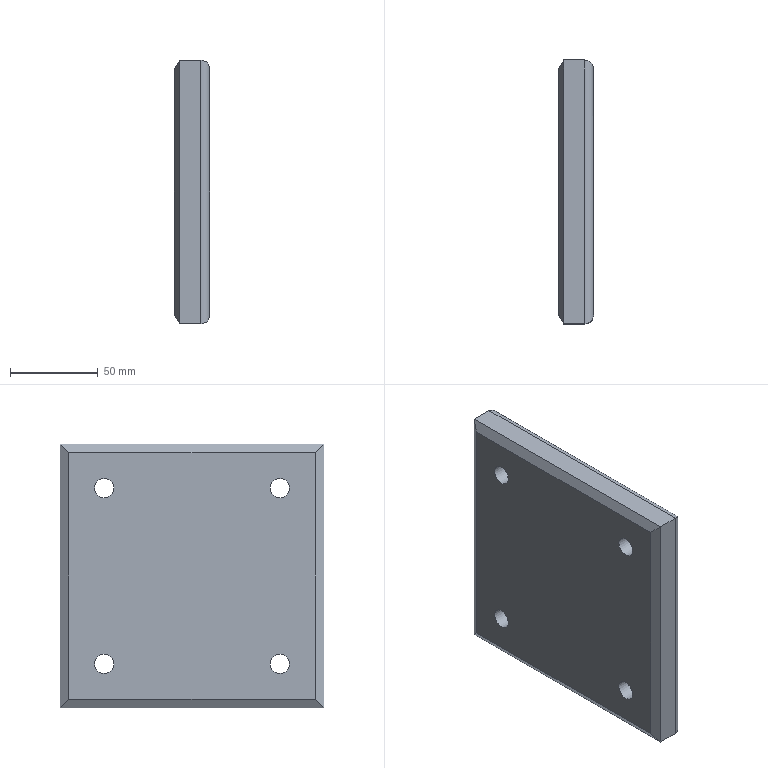Part | NX | features solid 2 | 1 solid | 30 faces | box 20 x 150 x 150 mm | volume 427385 mm3 | plane 14 | cylinder 12 | torus 4 | commonest cylinder face diameters 10 x4 11 x4 17.5 x4
STEP:
#1=CARTESIAN_POINT('',(715.,-50.,-145.));
#2=VERTEX_POINT('',#1);
#3=CARTESIAN_POINT('',(715.,-50.,-285.));
#4=VERTEX_POINT('',#3);
#5=CARTESIAN_POINT('',(715.,-50.,-290.));
#6=DIRECTION('',(0.,0.,-1.));
#7=VECTOR('',#6,1000.);
#8=LINE('',#5,#7);
#9=EDGE_CURVE('',#2,#4,#8,.T.);
#10=ORIENTED_EDGE('',*,*,#9,.F.);
#11=CARTESIAN_POINT('',(715.,-190.,-145.));
#12=VERTEX_POINT('',#11);
#13=CARTESIAN_POINT('',(715.,-195.,-145.));
#14=DIRECTION('',(0.,1.,0.));
#15=VECTOR('',#14,1000.);
#16=LINE('',#13,#15);
#17=EDGE_CURVE('',#12,#2,#16,.T.);
#18=ORIENTED_EDGE('',*,*,#17,.F.);
#19=CARTESIAN_POINT('',(715.,-190.,-285.));
#20=VERTEX_POINT('',#19);
#21=CARTESIAN_POINT('',(715.,-190.,-140.));
#22=DIRECTION('',(0.,0.,1.));
#23=VECTOR('',#22,1000.);
#24=LINE('',#21,#23);
#25=EDGE_CURVE('',#20,#12,#24,.T.);
#26=ORIENTED_EDGE('',*,*,#25,.F.);
#27=CARTESIAN_POINT('',(715.,-195.,-285.));
#28=DIRECTION('',(0.,-1.,0.));
#29=VECTOR('',#28,1000.);
#30=LINE('',#27,#29);
#31=EDGE_CURVE('',#4,#20,#30,.T.);
#32=ORIENTED_EDGE('',*,*,#31,.F.);
#33=EDGE_LOOP('',(#10,#18,#26,#32));
#34=FACE_BOUND('',#33,.T.);
#35=CARTESIAN_POINT('',(715.,-70.,-153.25));
#36=VERTEX_POINT('',#35);
#37=CARTESIAN_POINT('',(715.,-70.,-165.));
#38=DIRECTION('',(1.,0.,0.));
#39=DIRECTION('',(0.,0.,1.));
#40=AXIS2_PLACEMENT_3D('',#37,#38,#39);
#41=CIRCLE('',#40,11.75);
#42=EDGE_CURVE('',#36,#36,#41,.T.);
#43=ORIENTED_EDGE('',*,*,#42,.F.);
#44=EDGE_LOOP('',(#43));
#45=FACE_BOUND('',#44,.T.);
#46=CARTESIAN_POINT('',(715.,-70.,-253.25));
#47=VERTEX_POINT('',#46);
#48=CARTESIAN_POINT('',(715.,-70.,-265.));
#49=DIRECTION('',(1.,0.,0.));
#50=DIRECTION('',(0.,0.,1.));
#51=AXIS2_PLACEMENT_3D('',#48,#49,#50);
#52=CIRCLE('',#51,11.75);
#53=EDGE_CURVE('',#47,#47,#52,.T.);
#54=ORIENTED_EDGE('',*,*,#53,.F.);
#55=EDGE_LOOP('',(#54));
#56=FACE_BOUND('',#55,.T.);
#57=CARTESIAN_POINT('',(715.,-170.,-253.25));
#58=VERTEX_POINT('',#57);
#59=CARTESIAN_POINT('',(715.,-170.,-265.));
#60=DIRECTION('',(1.,0.,0.));
#61=DIRECTION('',(0.,0.,1.));
#62=AXIS2_PLACEMENT_3D('',#59,#60,#61);
#63=CIRCLE('',#62,11.75);
#64=EDGE_CURVE('',#58,#58,#63,.T.);
#65=ORIENTED_EDGE('',*,*,#64,.F.);
#66=EDGE_LOOP('',(#65));
#67=FACE_BOUND('',#66,.T.);
#68=CARTESIAN_POINT('',(715.,-170.,-153.25));
#69=VERTEX_POINT('',#68);
#70=CARTESIAN_POINT('',(715.,-170.,-165.));
#71=DIRECTION('',(1.,0.,0.));
#72=DIRECTION('',(0.,0.,1.));
#73=AXIS2_PLACEMENT_3D('',#70,#71,#72);
#74=CIRCLE('',#73,11.75);
#75=EDGE_CURVE('',#69,#69,#74,.T.);
#76=ORIENTED_EDGE('',*,*,#75,.F.);
#77=EDGE_LOOP('',(#76));
#78=FACE_BOUND('',#77,.T.);
#79=CARTESIAN_POINT('',(715.,-195.,-290.));
#80=DIRECTION('',(1.,0.,0.));
#81=DIRECTION('',(0.,0.,-1.));
#82=AXIS2_PLACEMENT_3D('',#79,#80,#81);
#83=PLANE('',#82);
#84=ADVANCED_FACE('',(#34,#45,#56,#67,#78),#83,.T.);
#85=CARTESIAN_POINT('',(710.,-195.,-140.));
#86=VERTEX_POINT('',#85);
#87=CARTESIAN_POINT('',(698.,-195.,-140.));
#88=VERTEX_POINT('',#87);
#89=CARTESIAN_POINT('',(715.,-195.,-140.));
#90=DIRECTION('',(-1.,0.,0.));
#91=VECTOR('',#90,1000.);
#92=LINE('',#89,#91);
#93=EDGE_CURVE('',#86,#88,#92,.T.);
#94=ORIENTED_EDGE('',*,*,#93,.F.);
#95=CARTESIAN_POINT('',(710.,-45.,-140.));
#96=VERTEX_POINT('',#95);
#97=CARTESIAN_POINT('',(710.,-195.,-140.));
#98=DIRECTION('',(0.,-1.,0.));
#99=VECTOR('',#98,1000.);
#100=LINE('',#97,#99);
#101=EDGE_CURVE('',#96,#86,#100,.T.);
#102=ORIENTED_EDGE('',*,*,#101,.F.);
#103=CARTESIAN_POINT('',(698.,-45.,-140.));
#104=VERTEX_POINT('',#103);
#105=CARTESIAN_POINT('',(715.,-45.,-140.));
#106=DIRECTION('',(-1.,0.,0.));
#107=VECTOR('',#106,1000.);
#108=LINE('',#105,#107);
#109=EDGE_CURVE('',#96,#104,#108,.T.);
#110=ORIENTED_EDGE('',*,*,#109,.T.);
#111=CARTESIAN_POINT('',(698.,-195.,-140.));
#112=DIRECTION('',(0.,1.,0.));
#113=VECTOR('',#112,1000.);
#114=LINE('',#111,#113);
#115=EDGE_CURVE('',#88,#104,#114,.T.);
#116=ORIENTED_EDGE('',*,*,#115,.F.);
#117=EDGE_LOOP('',(#94,#102,#110,#116));
#118=FACE_BOUND('',#117,.T.);
#119=CARTESIAN_POINT('',(715.,-195.,-140.));
#120=DIRECTION('',(0.,0.,1.));
#121=DIRECTION('',(1.,0.,0.));
#122=AXIS2_PLACEMENT_3D('',#119,#120,#121);
#123=PLANE('',#122);
#124=ADVANCED_FACE('',(#118),#123,.T.);
#125=CARTESIAN_POINT('',(695.,-190.,-145.));
#126=VERTEX_POINT('',#125);
#127=CARTESIAN_POINT('',(695.,-190.,-285.));
#128=VERTEX_POINT('',#127);
#129=CARTESIAN_POINT('',(695.,-190.,-290.));
#130=DIRECTION('',(0.,0.,-1.));
#131=VECTOR('',#130,1000.);
#132=LINE('',#129,#131);
#133=EDGE_CURVE('',#126,#128,#132,.T.);
#134=ORIENTED_EDGE('',*,*,#133,.F.);
#135=CARTESIAN_POINT('',(695.,-50.,-145.));
#136=VERTEX_POINT('',#135);
#137=CARTESIAN_POINT('',(695.,-195.,-145.));
#138=DIRECTION('',(0.,-1.,0.));
#139=VECTOR('',#138,1000.);
#140=LINE('',#137,#139);
#141=EDGE_CURVE('',#136,#126,#140,.T.);
#142=ORIENTED_EDGE('',*,*,#141,.F.);
#143=CARTESIAN_POINT('',(695.,-50.,-285.));
#144=VERTEX_POINT('',#143);
#145=CARTESIAN_POINT('',(695.,-50.,-290.));
#146=DIRECTION('',(0.,0.,1.));
#147=VECTOR('',#146,1000.);
#148=LINE('',#145,#147);
#149=EDGE_CURVE('',#144,#136,#148,.T.);
#150=ORIENTED_EDGE('',*,*,#149,.F.);
#151=CARTESIAN_POINT('',(695.,-195.,-285.));
#152=DIRECTION('',(0.,1.,0.));
#153=VECTOR('',#152,1000.);
#154=LINE('',#151,#153);
#155=EDGE_CURVE('',#128,#144,#154,.T.);
#156=ORIENTED_EDGE('',*,*,#155,.F.);
#157=EDGE_LOOP('',(#134,#142,#150,#156));
#158=FACE_BOUND('',#157,.T.);
#159=CARTESIAN_POINT('',(695.,-170.,-259.5));
#160=VERTEX_POINT('',#159);
#161=CARTESIAN_POINT('',(695.,-170.,-265.));
#162=DIRECTION('',(1.,0.,0.));
#163=DIRECTION('',(0.,0.,1.));
#164=AXIS2_PLACEMENT_3D('',#161,#162,#163);
#165=CIRCLE('',#164,5.5);
#166=EDGE_CURVE('',#160,#160,#165,.T.);
#167=ORIENTED_EDGE('',*,*,#166,.T.);
#168=EDGE_LOOP('',(#167));
#169=FACE_BOUND('',#168,.T.);
#170=CARTESIAN_POINT('',(695.,-70.,-259.5));
#171=VERTEX_POINT('',#170);
#172=CARTESIAN_POINT('',(695.,-70.,-265.));
#173=DIRECTION('',(1.,0.,0.));
#174=DIRECTION('',(0.,0.,1.));
#175=AXIS2_PLACEMENT_3D('',#172,#173,#174);
#176=CIRCLE('',#175,5.5);
#177=EDGE_CURVE('',#171,#171,#176,.T.);
#178=ORIENTED_EDGE('',*,*,#177,.T.);
#179=EDGE_LOOP('',(#178));
#180=FACE_BOUND('',#179,.T.);
#181=CARTESIAN_POINT('',(695.,-170.,-159.5));
#182=VERTEX_POINT('',#181);
#183=CARTESIAN_POINT('',(695.,-170.,-165.));
#184=DIRECTION('',(1.,0.,0.));
#185=DIRECTION('',(0.,0.,1.));
#186=AXIS2_PLACEMENT_3D('',#183,#184,#185);
#187=CIRCLE('',#186,5.5);
#188=EDGE_CURVE('',#182,#182,#187,.T.);
#189=ORIENTED_EDGE('',*,*,#188,.T.);
#190=EDGE_LOOP('',(#189));
#191=FACE_BOUND('',#190,.T.);
#192=CARTESIAN_POINT('',(695.,-70.,-159.5));
#193=VERTEX_POINT('',#192);
#194=CARTESIAN_POINT('',(695.,-70.,-165.));
#195=DIRECTION('',(1.,0.,0.));
#196=DIRECTION('',(0.,0.,1.));
#197=AXIS2_PLACEMENT_3D('',#194,#195,#196);
#198=CIRCLE('',#197,5.5);
#199=EDGE_CURVE('',#193,#193,#198,.T.);
#200=ORIENTED_EDGE('',*,*,#199,.T.);
#201=EDGE_LOOP('',(#200));
#202=FACE_BOUND('',#201,.T.);
#203=CARTESIAN_POINT('',(695.,-195.,-290.));
#204=DIRECTION('',(1.,0.,0.));
#205=DIRECTION('',(0.,0.,-1.));
#206=AXIS2_PLACEMENT_3D('',#203,#204,#205);
#207=PLANE('',#206);
#208=ADVANCED_FACE('',(#158,#169,#180,#191,#202),#207,.F.);
#209=CARTESIAN_POINT('',(710.,-45.,-290.));
#210=VERTEX_POINT('',#209);
#211=CARTESIAN_POINT('',(698.,-45.,-290.));
#212=VERTEX_POINT('',#211);
#213=CARTESIAN_POINT('',(715.,-45.,-290.));
#214=DIRECTION('',(-1.,0.,0.));
#215=VECTOR('',#214,1000.);
#216=LINE('',#213,#215);
#217=EDGE_CURVE('',#210,#212,#216,.T.);
#218=ORIENTED_EDGE('',*,*,#217,.F.);
#219=CARTESIAN_POINT('',(710.,-195.,-290.));
#220=VERTEX_POINT('',#219);
#221=CARTESIAN_POINT('',(710.,-195.,-290.));
#222=DIRECTION('',(0.,1.,0.));
#223=VECTOR('',#222,1000.);
#224=LINE('',#221,#223);
#225=EDGE_CURVE('',#220,#210,#224,.T.);
#226=ORIENTED_EDGE('',*,*,#225,.F.);
#227=CARTESIAN_POINT('',(698.,-195.,-290.));
#228=VERTEX_POINT('',#227);
#229=CARTESIAN_POINT('',(715.,-195.,-290.));
#230=DIRECTION('',(-1.,0.,0.));
#231=VECTOR('',#230,1000.);
#232=LINE('',#229,#231);
#233=EDGE_CURVE('',#220,#228,#232,.T.);
#234=ORIENTED_EDGE('',*,*,#233,.T.);
#235=CARTESIAN_POINT('',(698.,-195.,-290.));
#236=DIRECTION('',(0.,-1.,0.));
#237=VECTOR('',#236,1000.);
#238=LINE('',#235,#237);
#239=EDGE_CURVE('',#212,#228,#238,.T.);
#240=ORIENTED_EDGE('',*,*,#239,.F.);
#241=EDGE_LOOP('',(#218,#226,#234,#240));
#242=FACE_BOUND('',#241,.T.);
#243=CARTESIAN_POINT('',(715.,-195.,-290.));
#244=DIRECTION('',(0.,0.,1.));
#245=DIRECTION('',(1.,0.,0.));
#246=AXIS2_PLACEMENT_3D('',#243,#244,#245);
#247=PLANE('',#246);
#248=ADVANCED_FACE('',(#242),#247,.F.);
#249=ORIENTED_EDGE('',*,*,#109,.F.);
#250=CARTESIAN_POINT('',(710.,-45.,-290.));
#251=DIRECTION('',(0.,0.,1.));
#252=VECTOR('',#251,1000.);
#253=LINE('',#250,#252);
#254=EDGE_CURVE('',#210,#96,#253,.T.);
#255=ORIENTED_EDGE('',*,*,#254,.F.);
#256=ORIENTED_EDGE('',*,*,#217,.T.);
#257=CARTESIAN_POINT('',(698.,-45.,-290.));
#258=DIRECTION('',(0.,0.,-1.));
#259=VECTOR('',#258,1000.);
#260=LINE('',#257,#259);
#261=EDGE_CURVE('',#104,#212,#260,.T.);
#262=ORIENTED_EDGE('',*,*,#261,.F.);
#263=EDGE_LOOP('',(#249,#255,#256,#262));
#264=FACE_BOUND('',#263,.T.);
#265=CARTESIAN_POINT('',(715.,-45.,-290.));
#266=DIRECTION('',(0.,1.,0.));
#267=DIRECTION('',(0.,0.,-1.));
#268=AXIS2_PLACEMENT_3D('',#265,#266,#267);
#269=PLANE('',#268);
#270=ADVANCED_FACE('',(#264),#269,.T.);
#271=ORIENTED_EDGE('',*,*,#233,.F.);
#272=CARTESIAN_POINT('',(710.,-195.,-290.));
#273=DIRECTION('',(0.,0.,-1.));
#274=VECTOR('',#273,1000.);
#275=LINE('',#272,#274);
#276=EDGE_CURVE('',#86,#220,#275,.T.);
#277=ORIENTED_EDGE('',*,*,#276,.F.);
#278=ORIENTED_EDGE('',*,*,#93,.T.);
#279=CARTESIAN_POINT('',(698.,-195.,-140.));
#280=DIRECTION('',(0.,0.,1.));
#281=VECTOR('',#280,1000.);
#282=LINE('',#279,#281);
#283=EDGE_CURVE('',#228,#88,#282,.T.);
#284=ORIENTED_EDGE('',*,*,#283,.F.);
#285=EDGE_LOOP('',(#271,#277,#278,#284));
#286=FACE_BOUND('',#285,.T.);
#287=CARTESIAN_POINT('',(715.,-195.,-290.));
#288=DIRECTION('',(0.,1.,0.));
#289=DIRECTION('',(0.,0.,-1.));
#290=AXIS2_PLACEMENT_3D('',#287,#288,#289);
#291=PLANE('',#290);
#292=ADVANCED_FACE('',(#286),#291,.F.);
#293=ORIENTED_EDGE('',*,*,#199,.F.);
#294=EDGE_LOOP('',(#293));
#295=FACE_BOUND('',#294,.T.);
#296=CARTESIAN_POINT('',(703.,-70.,-170.5));
#297=VERTEX_POINT('',#296);
#298=CARTESIAN_POINT('',(703.,-70.,-165.));
#299=DIRECTION('',(1.,0.,0.));
#300=DIRECTION('',(0.,0.,-1.));
#301=AXIS2_PLACEMENT_3D('',#298,#299,#300);
#302=CIRCLE('',#301,5.5);
#303=EDGE_CURVE('',#297,#297,#302,.T.);
#304=ORIENTED_EDGE('',*,*,#303,.T.);
#305=EDGE_LOOP('',(#304));
#306=FACE_BOUND('',#305,.T.);
#307=CARTESIAN_POINT('',(665.,-70.,-165.));
#308=DIRECTION('',(-1.,0.,0.));
#309=DIRECTION('',(0.,0.,1.));
#310=AXIS2_PLACEMENT_3D('',#307,#308,#309);
#311=CYLINDRICAL_SURFACE('',#310,5.5);
#312=ADVANCED_FACE('',(#295,#306),#311,.F.);
#313=ORIENTED_EDGE('',*,*,#303,.F.);
#314=EDGE_LOOP('',(#313));
#315=FACE_BOUND('',#314,.T.);
#316=CARTESIAN_POINT('',(703.,-70.,-173.75));
#317=VERTEX_POINT('',#316);
#318=CARTESIAN_POINT('',(703.,-70.,-165.));
#319=DIRECTION('',(1.,0.,0.));
#320=DIRECTION('',(0.,0.,-1.));
#321=AXIS2_PLACEMENT_3D('',#318,#319,#320);
#322=CIRCLE('',#321,8.75);
#323=EDGE_CURVE('',#317,#317,#322,.T.);
#324=ORIENTED_EDGE('',*,*,#323,.T.);
#325=EDGE_LOOP('',(#324));
#326=FACE_BOUND('',#325,.T.);
#327=CARTESIAN_POINT('',(703.,-70.,-165.));
#328=DIRECTION('',(-1.,0.,0.));
#329=DIRECTION('',(0.,0.,1.));
#330=AXIS2_PLACEMENT_3D('',#327,#328,#329);
#331=PLANE('',#330);
#332=ADVANCED_FACE('',(#315,#326),#331,.F.);
#333=CARTESIAN_POINT('',(712.,-70.,-156.25));
#334=VERTEX_POINT('',#333);
#335=CARTESIAN_POINT('',(712.,-70.,-165.));
#336=DIRECTION('',(-1.,0.,0.));
#337=DIRECTION('',(0.,0.,1.));
#338=AXIS2_PLACEMENT_3D('',#335,#336,#337);
#339=CIRCLE('',#338,8.75);
#340=EDGE_CURVE('',#334,#334,#339,.T.);
#341=ORIENTED_EDGE('',*,*,#340,.F.);
#342=EDGE_LOOP('',(#341));
#343=FACE_BOUND('',#342,.T.);
#344=ORIENTED_EDGE('',*,*,#323,.F.);
#345=EDGE_LOOP('',(#344));
#346=FACE_BOUND('',#345,.T.);
#347=CARTESIAN_POINT('',(715.,-70.,-165.));
#348=DIRECTION('',(-1.,0.,0.));
#349=DIRECTION('',(0.,0.,1.));
#350=AXIS2_PLACEMENT_3D('',#347,#348,#349);
#351=CYLINDRICAL_SURFACE('',#350,8.75);
#352=ADVANCED_FACE('',(#343,#346),#351,.F.);
#353=ORIENTED_EDGE('',*,*,#188,.F.);
#354=EDGE_LOOP('',(#353));
#355=FACE_BOUND('',#354,.T.);
#356=CARTESIAN_POINT('',(703.,-170.,-170.5));
#357=VERTEX_POINT('',#356);
#358=CARTESIAN_POINT('',(703.,-170.,-165.));
#359=DIRECTION('',(1.,0.,0.));
#360=DIRECTION('',(0.,0.,-1.));
#361=AXIS2_PLACEMENT_3D('',#358,#359,#360);
#362=CIRCLE('',#361,5.5);
#363=EDGE_CURVE('',#357,#357,#362,.T.);
#364=ORIENTED_EDGE('',*,*,#363,.T.);
#365=EDGE_LOOP('',(#364));
#366=FACE_BOUND('',#365,.T.);
#367=CARTESIAN_POINT('',(665.,-170.,-165.));
#368=DIRECTION('',(-1.,0.,0.));
#369=DIRECTION('',(0.,0.,1.));
#370=AXIS2_PLACEMENT_3D('',#367,#368,#369);
#371=CYLINDRICAL_SURFACE('',#370,5.5);
#372=ADVANCED_FACE('',(#355,#366),#371,.F.);
#373=ORIENTED_EDGE('',*,*,#363,.F.);
#374=EDGE_LOOP('',(#373));
#375=FACE_BOUND('',#374,.T.);
#376=CARTESIAN_POINT('',(703.,-170.,-173.75));
#377=VERTEX_POINT('',#376);
#378=CARTESIAN_POINT('',(703.,-170.,-165.));
#379=DIRECTION('',(1.,0.,0.));
#380=DIRECTION('',(0.,0.,-1.));
#381=AXIS2_PLACEMENT_3D('',#378,#379,#380);
#382=CIRCLE('',#381,8.75);
#383=EDGE_CURVE('',#377,#377,#382,.T.);
#384=ORIENTED_EDGE('',*,*,#383,.T.);
#385=EDGE_LOOP('',(#384));
#386=FACE_BOUND('',#385,.T.);
#387=CARTESIAN_POINT('',(703.,-170.,-165.));
#388=DIRECTION('',(-1.,0.,0.));
#389=DIRECTION('',(0.,0.,1.));
#390=AXIS2_PLACEMENT_3D('',#387,#388,#389);
#391=PLANE('',#390);
#392=ADVANCED_FACE('',(#375,#386),#391,.F.);
#393=CARTESIAN_POINT('',(712.,-170.,-156.25));
#394=VERTEX_POINT('',#393);
#395=CARTESIAN_POINT('',(712.,-170.,-165.));
#396=DIRECTION('',(-1.,0.,0.));
#397=DIRECTION('',(0.,0.,1.));
#398=AXIS2_PLACEMENT_3D('',#395,#396,#397);
#399=CIRCLE('',#398,8.75);
#400=EDGE_CURVE('',#394,#394,#399,.T.);
#401=ORIENTED_EDGE('',*,*,#400,.F.);
#402=EDGE_LOOP('',(#401));
#403=FACE_BOUND('',#402,.T.);
#404=ORIENTED_EDGE('',*,*,#383,.F.);
#405=EDGE_LOOP('',(#404));
#406=FACE_BOUND('',#405,.T.);
#407=CARTESIAN_POINT('',(715.,-170.,-165.));
#408=DIRECTION('',(-1.,0.,0.));
#409=DIRECTION('',(0.,0.,1.));
#410=AXIS2_PLACEMENT_3D('',#407,#408,#409);
#411=CYLINDRICAL_SURFACE('',#410,8.75);
#412=ADVANCED_FACE('',(#403,#406),#411,.F.);
#413=ORIENTED_EDGE('',*,*,#177,.F.);
#414=EDGE_LOOP('',(#413));
#415=FACE_BOUND('',#414,.T.);
#416=CARTESIAN_POINT('',(703.,-70.,-270.5));
#417=VERTEX_POINT('',#416);
#418=CARTESIAN_POINT('',(703.,-70.,-265.));
#419=DIRECTION('',(1.,0.,0.));
#420=DIRECTION('',(0.,0.,-1.));
#421=AXIS2_PLACEMENT_3D('',#418,#419,#420);
#422=CIRCLE('',#421,5.5);
#423=EDGE_CURVE('',#417,#417,#422,.T.);
#424=ORIENTED_EDGE('',*,*,#423,.T.);
#425=EDGE_LOOP('',(#424));
#426=FACE_BOUND('',#425,.T.);
#427=CARTESIAN_POINT('',(665.,-70.,-265.));
#428=DIRECTION('',(-1.,0.,0.));
#429=DIRECTION('',(0.,0.,1.));
#430=AXIS2_PLACEMENT_3D('',#427,#428,#429);
#431=CYLINDRICAL_SURFACE('',#430,5.5);
#432=ADVANCED_FACE('',(#415,#426),#431,.F.);
#433=ORIENTED_EDGE('',*,*,#423,.F.);
#434=EDGE_LOOP('',(#433));
#435=FACE_BOUND('',#434,.T.);
#436=CARTESIAN_POINT('',(703.,-70.,-273.75));
#437=VERTEX_POINT('',#436);
#438=CARTESIAN_POINT('',(703.,-70.,-265.));
#439=DIRECTION('',(1.,0.,0.));
#440=DIRECTION('',(0.,0.,-1.));
#441=AXIS2_PLACEMENT_3D('',#438,#439,#440);
#442=CIRCLE('',#441,8.75);
#443=EDGE_CURVE('',#437,#437,#442,.T.);
#444=ORIENTED_EDGE('',*,*,#443,.T.);
#445=EDGE_LOOP('',(#444));
#446=FACE_BOUND('',#445,.T.);
#447=CARTESIAN_POINT('',(703.,-70.,-265.));
#448=DIRECTION('',(-1.,0.,0.));
#449=DIRECTION('',(0.,0.,1.));
#450=AXIS2_PLACEMENT_3D('',#447,#448,#449);
#451=PLANE('',#450);
#452=ADVANCED_FACE('',(#435,#446),#451,.F.);
#453=CARTESIAN_POINT('',(712.,-70.,-256.25));
#454=VERTEX_POINT('',#453);
#455=CARTESIAN_POINT('',(712.,-70.,-265.));
#456=DIRECTION('',(-1.,0.,0.));
#457=DIRECTION('',(0.,0.,1.));
#458=AXIS2_PLACEMENT_3D('',#455,#456,#457);
#459=CIRCLE('',#458,8.75);
#460=EDGE_CURVE('',#454,#454,#459,.T.);
#461=ORIENTED_EDGE('',*,*,#460,.F.);
#462=EDGE_LOOP('',(#461));
#463=FACE_BOUND('',#462,.T.);
#464=ORIENTED_EDGE('',*,*,#443,.F.);
#465=EDGE_LOOP('',(#464));
#466=FACE_BOUND('',#465,.T.);
#467=CARTESIAN_POINT('',(715.,-70.,-265.));
#468=DIRECTION('',(-1.,0.,0.));
#469=DIRECTION('',(0.,0.,1.));
#470=AXIS2_PLACEMENT_3D('',#467,#468,#469);
#471=CYLINDRICAL_SURFACE('',#470,8.75);
#472=ADVANCED_FACE('',(#463,#466),#471,.F.);
#473=ORIENTED_EDGE('',*,*,#166,.F.);
#474=EDGE_LOOP('',(#473));
#475=FACE_BOUND('',#474,.T.);
#476=CARTESIAN_POINT('',(703.,-170.,-270.5));
#477=VERTEX_POINT('',#476);
#478=CARTESIAN_POINT('',(703.,-170.,-265.));
#479=DIRECTION('',(1.,0.,0.));
#480=DIRECTION('',(0.,0.,-1.));
#481=AXIS2_PLACEMENT_3D('',#478,#479,#480);
#482=CIRCLE('',#481,5.5);
#483=EDGE_CURVE('',#477,#477,#482,.T.);
#484=ORIENTED_EDGE('',*,*,#483,.T.);
#485=EDGE_LOOP('',(#484));
#486=FACE_BOUND('',#485,.T.);
#487=CARTESIAN_POINT('',(665.,-170.,-265.));
#488=DIRECTION('',(-1.,0.,0.));
#489=DIRECTION('',(0.,0.,1.));
#490=AXIS2_PLACEMENT_3D('',#487,#488,#489);
#491=CYLINDRICAL_SURFACE('',#490,5.5);
#492=ADVANCED_FACE('',(#475,#486),#491,.F.);
#493=ORIENTED_EDGE('',*,*,#483,.F.);
#494=EDGE_LOOP('',(#493));
#495=FACE_BOUND('',#494,.T.);
#496=CARTESIAN_POINT('',(703.,-170.,-273.75));
#497=VERTEX_POINT('',#496);
#498=CARTESIAN_POINT('',(703.,-170.,-265.));
#499=DIRECTION('',(1.,0.,0.));
#500=DIRECTION('',(0.,0.,-1.));
#501=AXIS2_PLACEMENT_3D('',#498,#499,#500);
#502=CIRCLE('',#501,8.75);
#503=EDGE_CURVE('',#497,#497,#502,.T.);
#504=ORIENTED_EDGE('',*,*,#503,.T.);
#505=EDGE_LOOP('',(#504));
#506=FACE_BOUND('',#505,.T.);
#507=CARTESIAN_POINT('',(703.,-170.,-265.));
#508=DIRECTION('',(-1.,0.,0.));
#509=DIRECTION('',(0.,0.,1.));
#510=AXIS2_PLACEMENT_3D('',#507,#508,#509);
#511=PLANE('',#510);
#512=ADVANCED_FACE('',(#495,#506),#511,.F.);
#513=CARTESIAN_POINT('',(712.,-170.,-256.25));
#514=VERTEX_POINT('',#513);
#515=CARTESIAN_POINT('',(712.,-170.,-265.));
#516=DIRECTION('',(-1.,0.,0.));
#517=DIRECTION('',(0.,0.,1.));
#518=AXIS2_PLACEMENT_3D('',#515,#516,#517);
#519=CIRCLE('',#518,8.75);
#520=EDGE_CURVE('',#514,#514,#519,.T.);
#521=ORIENTED_EDGE('',*,*,#520,.F.);
#522=EDGE_LOOP('',(#521));
#523=FACE_BOUND('',#522,.T.);
#524=ORIENTED_EDGE('',*,*,#503,.F.);
#525=EDGE_LOOP('',(#524));
#526=FACE_BOUND('',#525,.T.);
#527=CARTESIAN_POINT('',(715.,-170.,-265.));
#528=DIRECTION('',(-1.,0.,0.));
#529=DIRECTION('',(0.,0.,1.));
#530=AXIS2_PLACEMENT_3D('',#527,#528,#529);
#531=CYLINDRICAL_SURFACE('',#530,8.75);
#532=ADVANCED_FACE('',(#523,#526),#531,.F.);
#533=ORIENTED_EDGE('',*,*,#340,.T.);
#534=EDGE_LOOP('',(#533));
#535=FACE_BOUND('',#534,.T.);
#536=ORIENTED_EDGE('',*,*,#42,.T.);
#537=EDGE_LOOP('',(#536));
#538=FACE_BOUND('',#537,.T.);
#539=CARTESIAN_POINT('',(712.,-70.,-165.));
#540=DIRECTION('',(1.,0.,0.));
#541=DIRECTION('',(0.,0.,-1.));
#542=AXIS2_PLACEMENT_3D('',#539,#540,#541);
#543=TOROIDAL_SURFACE('',#542,11.75,3.);
#544=ADVANCED_FACE('',(#535,#538),#543,.T.);
#545=ORIENTED_EDGE('',*,*,#460,.T.);
#546=EDGE_LOOP('',(#545));
#547=FACE_BOUND('',#546,.T.);
#548=ORIENTED_EDGE('',*,*,#53,.T.);
#549=EDGE_LOOP('',(#548));
#550=FACE_BOUND('',#549,.T.);
#551=CARTESIAN_POINT('',(712.,-70.,-265.));
#552=DIRECTION('',(1.,0.,0.));
#553=DIRECTION('',(0.,0.,-1.));
#554=AXIS2_PLACEMENT_3D('',#551,#552,#553);
#555=TOROIDAL_SURFACE('',#554,11.75,3.);
#556=ADVANCED_FACE('',(#547,#550),#555,.T.);
#557=ORIENTED_EDGE('',*,*,#520,.T.);
#558=EDGE_LOOP('',(#557));
#559=FACE_BOUND('',#558,.T.);
#560=ORIENTED_EDGE('',*,*,#64,.T.);
#561=EDGE_LOOP('',(#560));
#562=FACE_BOUND('',#561,.T.);
#563=CARTESIAN_POINT('',(712.,-170.,-265.));
#564=DIRECTION('',(1.,0.,0.));
#565=DIRECTION('',(0.,0.,-1.));
#566=AXIS2_PLACEMENT_3D('',#563,#564,#565);
#567=TOROIDAL_SURFACE('',#566,11.75,3.);
#568=ADVANCED_FACE('',(#559,#562),#567,.T.);
#569=ORIENTED_EDGE('',*,*,#400,.T.);
#570=EDGE_LOOP('',(#569));
#571=FACE_BOUND('',#570,.T.);
#572=ORIENTED_EDGE('',*,*,#75,.T.);
#573=EDGE_LOOP('',(#572));
#574=FACE_BOUND('',#573,.T.);
#575=CARTESIAN_POINT('',(712.,-170.,-165.));
#576=DIRECTION('',(1.,0.,0.));
#577=DIRECTION('',(0.,0.,-1.));
#578=AXIS2_PLACEMENT_3D('',#575,#576,#577);
#579=TOROIDAL_SURFACE('',#578,11.75,3.);
#580=ADVANCED_FACE('',(#571,#574),#579,.T.);
#581=CARTESIAN_POINT('',(710.,-50.,-145.));
#582=DIRECTION('',(0.,-0.7071,0.7071));
#583=DIRECTION('',(0.,0.7071,0.7071));
#584=AXIS2_PLACEMENT_3D('',#581,#582,#583);
#585=ELLIPSE('',#584,7.071,5.);
#586=EDGE_CURVE('',#2,#96,#585,.T.);
#587=ORIENTED_EDGE('',*,*,#586,.T.);
#588=ORIENTED_EDGE('',*,*,#101,.T.);
#589=CARTESIAN_POINT('',(710.,-190.,-145.));
#590=DIRECTION('',(0.,0.7071,0.7071));
#591=DIRECTION('',(0.,0.7071,-0.7071));
#592=AXIS2_PLACEMENT_3D('',#589,#590,#591);
#593=ELLIPSE('',#592,7.071,5.);
#594=EDGE_CURVE('',#86,#12,#593,.T.);
#595=ORIENTED_EDGE('',*,*,#594,.T.);
#596=ORIENTED_EDGE('',*,*,#17,.T.);
#597=EDGE_LOOP('',(#587,#588,#595,#596));
#598=FACE_BOUND('',#597,.T.);
#599=CARTESIAN_POINT('',(710.,-195.,-145.));
#600=DIRECTION('',(0.,1.,0.));
#601=DIRECTION('',(0.,0.,-1.));
#602=AXIS2_PLACEMENT_3D('',#599,#600,#601);
#603=CYLINDRICAL_SURFACE('',#602,5.);
#604=ADVANCED_FACE('',(#598),#603,.T.);
#605=ORIENTED_EDGE('',*,*,#594,.F.);
#606=ORIENTED_EDGE('',*,*,#276,.T.);
#607=CARTESIAN_POINT('',(710.,-190.,-285.));
#608=DIRECTION('',(0.,-0.7071,0.7071));
#609=DIRECTION('',(0.,-0.7071,-0.7071));
#610=AXIS2_PLACEMENT_3D('',#607,#608,#609);
#611=ELLIPSE('',#610,7.071,5.);
#612=EDGE_CURVE('',#220,#20,#611,.T.);
#613=ORIENTED_EDGE('',*,*,#612,.T.);
#614=ORIENTED_EDGE('',*,*,#25,.T.);
#615=EDGE_LOOP('',(#605,#606,#613,#614));
#616=FACE_BOUND('',#615,.T.);
#617=CARTESIAN_POINT('',(710.,-190.,-290.));
#618=DIRECTION('',(0.,0.,-1.));
#619=DIRECTION('',(-1.,0.,0.));
#620=AXIS2_PLACEMENT_3D('',#617,#618,#619);
#621=CYLINDRICAL_SURFACE('',#620,5.);
#622=ADVANCED_FACE('',(#616),#621,.T.);
#623=ORIENTED_EDGE('',*,*,#586,.F.);
#624=ORIENTED_EDGE('',*,*,#9,.T.);
#625=CARTESIAN_POINT('',(710.,-50.,-285.));
#626=DIRECTION('',(0.,0.7071,0.7071));
#627=DIRECTION('',(0.,-0.7071,0.7071));
#628=AXIS2_PLACEMENT_3D('',#625,#626,#627);
#629=ELLIPSE('',#628,7.071,5.);
#630=EDGE_CURVE('',#4,#210,#629,.T.);
#631=ORIENTED_EDGE('',*,*,#630,.T.);
#632=ORIENTED_EDGE('',*,*,#254,.T.);
#633=EDGE_LOOP('',(#623,#624,#631,#632));
#634=FACE_BOUND('',#633,.T.);
#635=CARTESIAN_POINT('',(710.,-50.,-290.));
#636=DIRECTION('',(0.,0.,1.));
#637=DIRECTION('',(1.,0.,0.));
#638=AXIS2_PLACEMENT_3D('',#635,#636,#637);
#639=CYLINDRICAL_SURFACE('',#638,5.);
#640=ADVANCED_FACE('',(#634),#639,.T.);
#641=ORIENTED_EDGE('',*,*,#612,.F.);
#642=ORIENTED_EDGE('',*,*,#225,.T.);
#643=ORIENTED_EDGE('',*,*,#630,.F.);
#644=ORIENTED_EDGE('',*,*,#31,.T.);
#645=EDGE_LOOP('',(#641,#642,#643,#644));
#646=FACE_BOUND('',#645,.T.);
#647=CARTESIAN_POINT('',(710.,-195.,-285.));
#648=DIRECTION('',(0.,-1.,0.));
#649=DIRECTION('',(0.,0.,1.));
#650=AXIS2_PLACEMENT_3D('',#647,#648,#649);
#651=CYLINDRICAL_SURFACE('',#650,5.);
#652=ADVANCED_FACE('',(#646),#651,.T.);
#653=CARTESIAN_POINT('',(659.864,-108.559,-203.559));
#654=DIRECTION('',(-0.3906,-0.6509,-0.6509));
#655=VECTOR('',#654,1000.);
#656=LINE('',#653,#655);
#657=EDGE_CURVE('',#104,#136,#656,.T.);
#658=ORIENTED_EDGE('',*,*,#657,.T.);
#659=ORIENTED_EDGE('',*,*,#141,.T.);
#660=CARTESIAN_POINT('',(698.,-195.,-140.));
#661=DIRECTION('',(0.3906,-0.6509,0.6509));
#662=VECTOR('',#661,1000.);
#663=LINE('',#660,#662);
#664=EDGE_CURVE('',#126,#88,#663,.T.);
#665=ORIENTED_EDGE('',*,*,#664,.T.);
#666=ORIENTED_EDGE('',*,*,#115,.T.);
#667=EDGE_LOOP('',(#658,#659,#665,#666));
#668=FACE_BOUND('',#667,.T.);
#669=CARTESIAN_POINT('',(698.,-195.,-140.));
#670=DIRECTION('',(-0.8575,0.,0.5145));
#671=DIRECTION('',(0.5145,0.,0.8575));
#672=AXIS2_PLACEMENT_3D('',#669,#670,#671);
#673=PLANE('',#672);
#674=ADVANCED_FACE('',(#668),#673,.T.);
#675=ORIENTED_EDGE('',*,*,#664,.F.);
#676=ORIENTED_EDGE('',*,*,#133,.T.);
#677=CARTESIAN_POINT('',(698.,-195.,-290.));
#678=DIRECTION('',(0.3906,-0.6509,-0.6509));
#679=VECTOR('',#678,1000.);
#680=LINE('',#677,#679);
#681=EDGE_CURVE('',#128,#228,#680,.T.);
#682=ORIENTED_EDGE('',*,*,#681,.T.);
#683=ORIENTED_EDGE('',*,*,#283,.T.);
#684=EDGE_LOOP('',(#675,#676,#682,#683));
#685=FACE_BOUND('',#684,.T.);
#686=CARTESIAN_POINT('',(698.,-195.,-290.));
#687=DIRECTION('',(0.8575,0.5145,0.));
#688=DIRECTION('',(-0.5145,0.8575,0.));
#689=AXIS2_PLACEMENT_3D('',#686,#687,#688);
#690=PLANE('',#689);
#691=ADVANCED_FACE('',(#685),#690,.F.);
#692=ORIENTED_EDGE('',*,*,#657,.F.);
#693=ORIENTED_EDGE('',*,*,#261,.T.);
#694=CARTESIAN_POINT('',(696.271,-47.881,-287.119));
#695=DIRECTION('',(-0.3906,-0.6509,0.6509));
#696=VECTOR('',#695,1000.);
#697=LINE('',#694,#696);
#698=EDGE_CURVE('',#212,#144,#697,.T.);
#699=ORIENTED_EDGE('',*,*,#698,.T.);
#700=ORIENTED_EDGE('',*,*,#149,.T.);
#701=EDGE_LOOP('',(#692,#693,#699,#700));
#702=FACE_BOUND('',#701,.T.);
#703=CARTESIAN_POINT('',(695.,-50.,-290.));
#704=DIRECTION('',(-0.8575,0.5145,0.));
#705=DIRECTION('',(-0.5145,-0.8575,0.));
#706=AXIS2_PLACEMENT_3D('',#703,#704,#705);
#707=PLANE('',#706);
#708=ADVANCED_FACE('',(#702),#707,.T.);
#709=ORIENTED_EDGE('',*,*,#681,.F.);
#710=ORIENTED_EDGE('',*,*,#155,.T.);
#711=ORIENTED_EDGE('',*,*,#698,.F.);
#712=ORIENTED_EDGE('',*,*,#239,.T.);
#713=EDGE_LOOP('',(#709,#710,#711,#712));
#714=FACE_BOUND('',#713,.T.);
#715=CARTESIAN_POINT('',(695.,-195.,-285.));
#716=DIRECTION('',(0.8575,0.,0.5145));
#717=DIRECTION('',(0.5145,0.,-0.8575));
#718=AXIS2_PLACEMENT_3D('',#715,#716,#717);
#719=PLANE('',#718);
#720=ADVANCED_FACE('',(#714),#719,.F.);
#721=CLOSED_SHELL('',(#84,#124,#208,#248,#270,#292,#312,#332,#352,#372,#392,#412,#432,#452,#472,#492,#512,#532,#544,#556,#568,#580,#604,#622,#640,#652,#674,#691,#708,#720));
#722=MANIFOLD_SOLID_BREP('',#721);
#723=(LENGTH_UNIT()NAMED_UNIT(*)SI_UNIT(.MILLI.,.METRE.));
#724=UNCERTAINTY_MEASURE_WITH_UNIT(LENGTH_MEASURE(0.00001),#723,'','');
#725=(NAMED_UNIT(*)PLANE_ANGLE_UNIT()SI_UNIT($,.RADIAN.));
#726=(NAMED_UNIT(*)SI_UNIT($,.STERADIAN.)SOLID_ANGLE_UNIT());
#727=(GEOMETRIC_REPRESENTATION_CONTEXT(3)GLOBAL_UNCERTAINTY_ASSIGNED_CONTEXT((#724))GLOBAL_UNIT_ASSIGNED_CONTEXT((#723,#725,#726))REPRESENTATION_CONTEXT('',''));
#728=ADVANCED_BREP_SHAPE_REPRESENTATION('',(#722),#727);